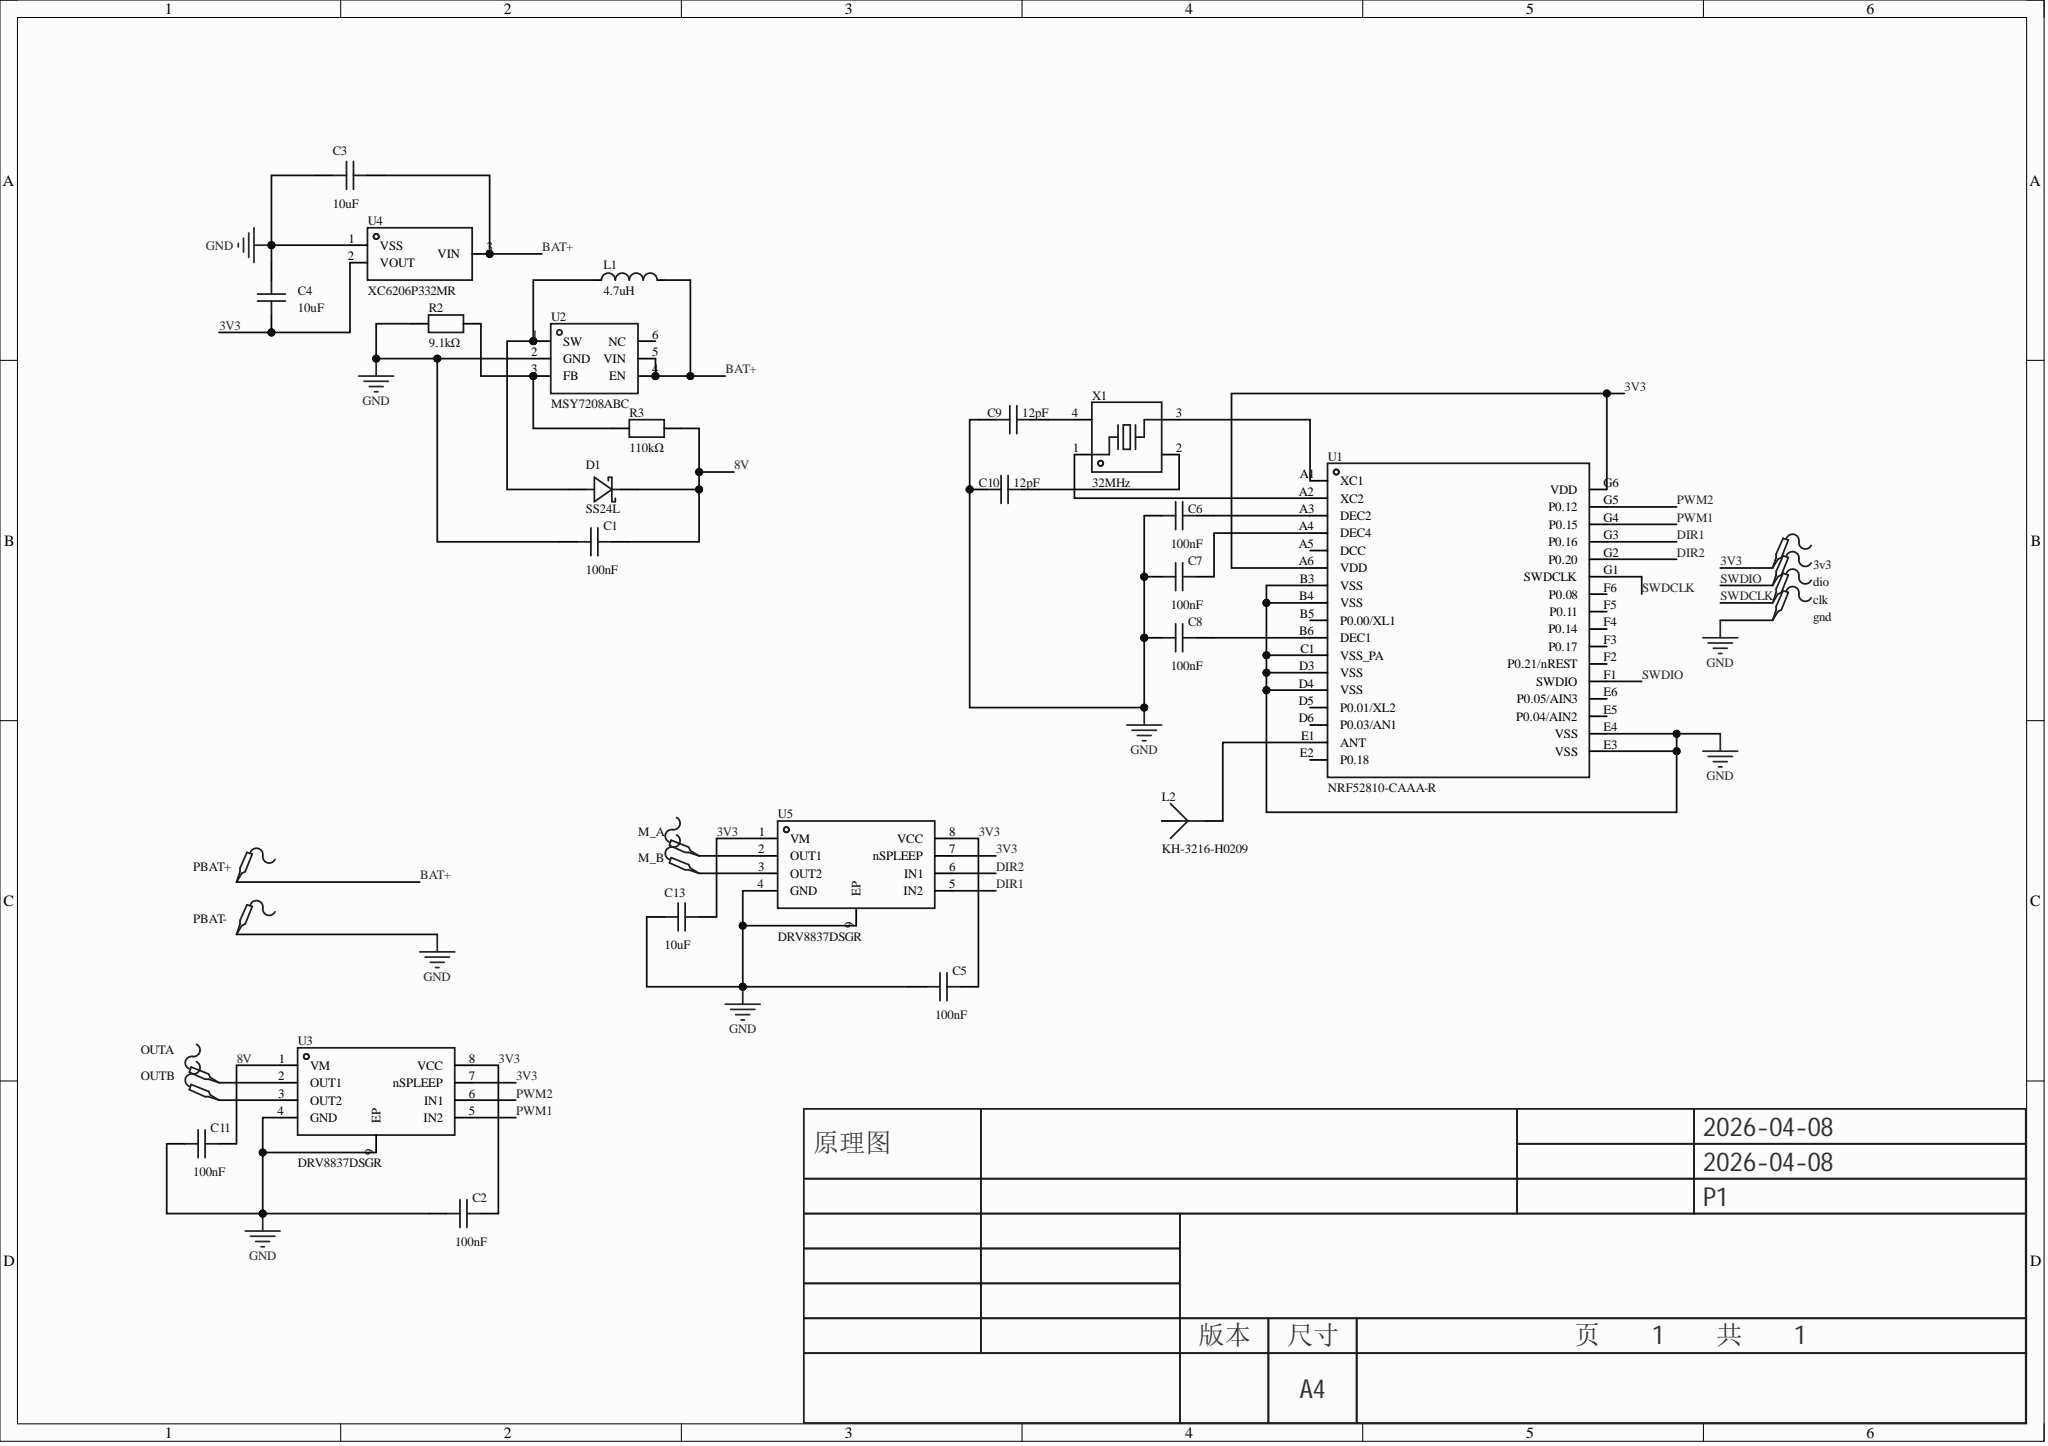Circuit board | Altium Designer | 33 parts | 24 nets
Bill of materials:
Comment,Description,Designator,Footprint,LibRef,Quantity
"","Test Point 测试点","3v3, clk, dio, gnd, M_A, M_B, OUTA, OUTB, PBAT-, PBAT+","Test-Point-0.5mm","Test-Point","10"
"100nF","容值:100nF;精度:±10%;额定电压:16V;温度系数:X7R;","C1, C2, C5, C6, C7, C8, C11","C0402","CL05B104KO5NNNC","7"
"10uF","容值:10uF;精度:±20%;额定电压:10V;温度系数:X5R;","C3, C4, C13","C0402","CGA0402X5R106M100GT","3"
"12pF","容值:12pF;精度:±5%;额定电压:50V;温度系数:C0G;","C9, C10","C0402","CGA0402C0G120J500GT","2"
"SS24L","二极管配置:独立式;正向压降(Vf):500mV@2A;直流反向耐压(Vr):40V;整流电流:2A;","D1","SOD-123FL_L2.8-W1.8-LS3.7-R-RD","SS24L_C2827931","1"
"4.7uH","电感值:4.7uH;精度:±20%;饱和电流(Isat):1.1A;","L1","IND-SMD_L2.5-W2.0_VLS2520X","VLS252012CX-4R7M","1"
"KH-3216-H0209","天线类型:贴片天线;中心频率:2.45GHz;带宽:120MHz;增益:1.71dBi;功率:4W;","L2","ANT-SMD_L3.2-W1.6-KH-3216F245C04","KH-3216-H0209","1"
"9.1kΩ","","R2","R0402","FRC0402F9101TS","1"
"110kΩ","","R3","R0402","FRC0402F1103TS","1"
"NRF52810-CAAA-R","频率范围:-;接口类型:ADC；PWM；UART；PDM；SPI;应用领域:蓝牙;数据速率:2Mbps;灵敏度:-96dBm;典型应用频率:2.4GHz;","U1","WLCSP-33_L2.5-W2.5-P0.40_NRF52810-CAAA-R","NRF52810-CAAA-R","1"
"MSY7208ABC","功能类型:升压型;工作电压:2.5V~24V;输出类型:可调;","U2","SOT-23-6_L2.9-W1.6-P0.95-LS2.8-BR","MSY7208ABC","1"
"DRV8837DSGR","DRV8837 12V、1.8A H 桥电机驱动器","U3, U5","WSON-8_L2.0-W2.0-P0.50-TL-EP","DRV8837DSGR","2"
"XC6206P332MR","输出类型:固定;工作电压:8V;输出电压:3.3V;输出电流:250mA;电源纹波抑制比(PSRR):40dB@(1kHz);输出极性:正极;","U4","SOT-23-3_L3.0-W1.7-P0.95-LS2.9-BR","XC6206P332MR_C347376","1"
"32MHz","晶振类型:贴片晶振;频率:32MHz;常温频差:±10ppm;负载电容:8pF;频率稳定度:±20ppm;","X1","CRYSTAL-SMD_4P-L2.0-W1.6-BL","XL7EL89CKI-111YLC-32M","1"
Netlist (Protel format):
[
3v3
Test-Point-0.5mm




]
[
C1
C0402
100nF



]
[
C2
C0402
100nF



]
[
C3
C0402
10uF



]
[
C4
C0402
10uF



]
[
C5
C0402
100nF



]
[
C6
C0402
100nF



]
[
C7
C0402
100nF



]
[
C8
C0402
100nF



]
[
C9
C0402
12pF



]
[
C10
C0402
12pF



]
[
C11
C0402
100nF



]
[
C13
C0402
10uF



]
[
clk
Test-Point-0.5mm




]
[
D1
SOD-123FL_L2.8-W1.8-LS3.7-R-RD
SS24L



]
[
dio
Test-Point-0.5mm




]
[
gnd
Test-Point-0.5mm




]
[
L1
IND-SMD_L2.5-W2.0_VLS2520X
4.7uH



]
[
L2
ANT-SMD_L3.2-W1.6-KH-3216F245C04
KH-3216-H0209



]
[
M_A
Test-Point-0.5mm




]
[
M_B
Test-Point-0.5mm




]
[
OUTA
Test-Point-0.5mm




]
[
OUTB
Test-Point-0.5mm




]
[
PBAT+
Test-Point-0.5mm




]
[
PBAT-
Test-Point-0.5mm




]
[
R2
R0402
9.1kΩ



]
[
R3
R0402
110kΩ



]
[
U1
WLCSP-33_L2.5-W2.5-P0.40_NRF52810-CAAA-R
NRF52810-CAAA-R



]
[
U2
SOT-23-6_L2.9-W1.6-P0.95-LS2.8-BR
MSY7208ABC



]
[
U3
WSON-8_L2.0-W2.0-P0.50-TL-EP
DRV8837DSGR



]
[
U4
SOT-23-3_L3.0-W1.7-P0.95-LS2.9-BR
XC6206P332MR



]
[
U5
WSON-8_L2.0-W2.0-P0.50-TL-EP
DRV8837DSGR



]
[
X1
CRYSTAL-SMD_4P-L2.0-W1.6-BL
32MHz



]
(
SWDIO
dio-1
U1-F1
)
(
SWDCLK
clk-1
U1-G1
)
(
PWM2
U1-G5
U3-6
)
(
PWM1
U1-G4
U3-5
)
(
NetU1_A2
U1-A2
X1-1
)
(
NetU1_A1
U1-A1
X1-3
)
(
NetR2_2
R2-2
R3-1
U2-3
)
(
NetOUTB_1
OUTB-1
U3-3
)
(
NetOUTA_1
OUTA-1
U3-2
)
(
NetM_B_1
M_B-1
U5-3
)
(
NetM_A_1
M_A-1
U5-2
)
(
NetL2_1
L2-1
U1-E1
)
(
NetD1_1
D1-1
L1-1
U2-1
)
(
NetC10_2
C10-2
X1-2
)
(
NetC9_2
C9-2
X1-4
)
(
NetC8_2
C8-2
U1-B6
)
(
NetC7_2
C7-2
U1-A4
)
(
NetC6_2
C6-2
U1-A3
)
(
GND
C1-1
C2-1
C3-1
C4-2
C5-1
C6-1
C7-1
C8-1
C9-1
C10-1
C11-1
C13-2
gnd-1
PBAT--1
R2-1
U1-B3
U1-B4
U1-C1
U1-D3
U1-D4
U1-E3
U1-E4
U2-2
U3-4
U3-9
U4-1
U5-4
U5-9
)
(
DIR2
U1-G2
U5-6
)
(
DIR1
U1-G3
U5-5
)
(
BAT+
C3-2
L1-2
PBAT+-1
U2-4
U2-5
U4-3
)
(
8V
C1-2
C11-2
D1-2
R3-2
U3-1
)
(
3V3
3v3-1
C2-2
C4-1
C5-2
C13-1
U1-A6
U1-G6
U3-7
U3-8
U4-2
U5-1
U5-7
U5-8
)